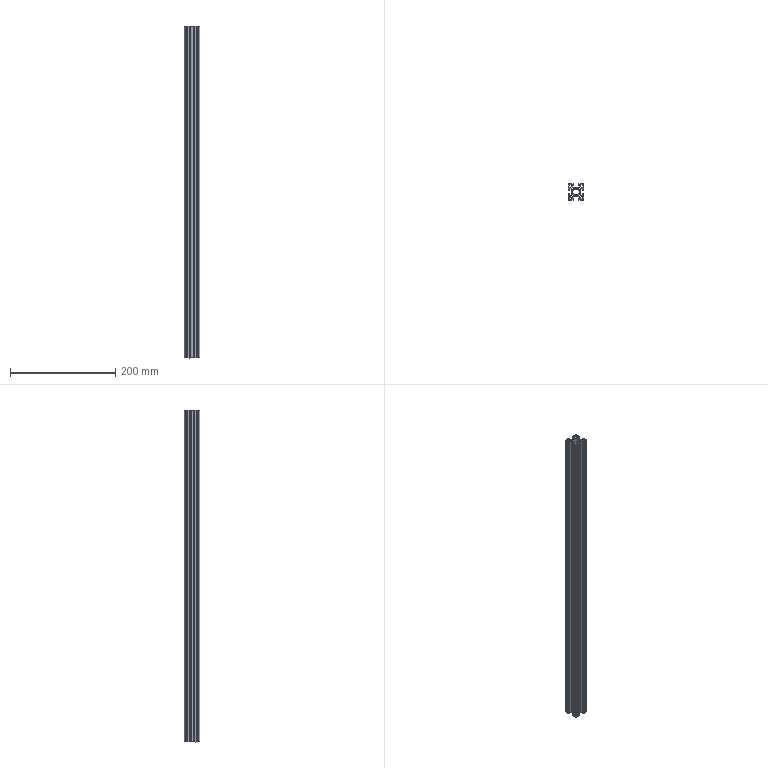Part | STEP file | 3030 printer light curtain mount | 1 solid | 154 faces | box 29.915 x 30.09 x 629.59 mm | volume 197400 mm3 | plane 110 | cylinder 44 | commonest cylinder face diameters 2 x15 4 x14 5 x8 16 x5 12 x2